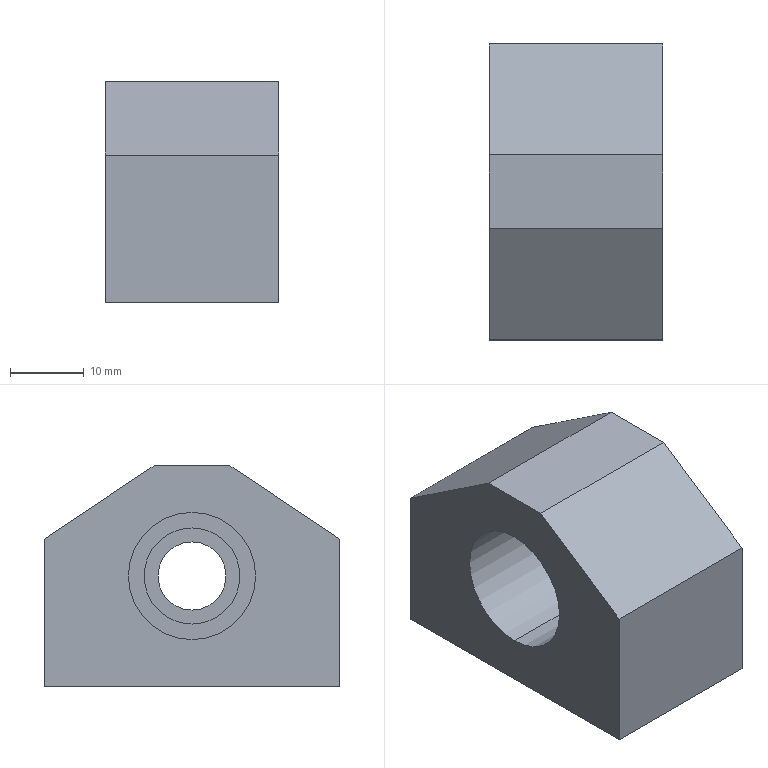Part | SolidWorks | features BaseBody 1 | 1 solid | 22 faces | box 23.5 x 40 x 30 mm | volume 19711 mm3 | plane 12 | cylinder 10 | commonest cylinder face diameters 6 x4 9.2 x2 13 x2 17.2 x2
STEP:
#1=CARTESIAN_POINT('',(896.946,-4295.973,955.371));
#2=VERTEX_POINT('',#1);
#3=CARTESIAN_POINT('',(896.946,-4295.973,964.571));
#4=VERTEX_POINT('',#3);
#5=CARTESIAN_POINT('',(896.946,-4295.973,959.971));
#6=DIRECTION('',(-1.,0.,0.));
#7=DIRECTION('',(0.,0.,1.));
#8=AXIS2_PLACEMENT_3D('',#5,#6,#7);
#9=CIRCLE('',#8,4.6);
#10=EDGE_CURVE('',#2,#4,#9,.T.);
#11=ORIENTED_EDGE('',*,*,#10,.F.);
#12=CARTESIAN_POINT('',(893.946,-4295.973,955.371));
#13=VERTEX_POINT('',#12);
#14=CARTESIAN_POINT('',(851.713,-4295.973,955.371));
#15=DIRECTION('',(-1.,0.,0.));
#16=VECTOR('',#15,1000.);
#17=LINE('',#14,#16);
#18=EDGE_CURVE('',#2,#13,#17,.T.);
#19=ORIENTED_EDGE('',*,*,#18,.T.);
#20=CARTESIAN_POINT('',(893.946,-4295.973,964.571));
#21=VERTEX_POINT('',#20);
#22=CARTESIAN_POINT('',(893.946,-4295.973,959.971));
#23=DIRECTION('',(1.,0.,0.));
#24=DIRECTION('',(0.,0.,1.));
#25=AXIS2_PLACEMENT_3D('',#22,#23,#24);
#26=CIRCLE('',#25,4.6);
#27=EDGE_CURVE('',#21,#13,#26,.T.);
#28=ORIENTED_EDGE('',*,*,#27,.F.);
#29=CARTESIAN_POINT('',(851.713,-4295.973,964.571));
#30=DIRECTION('',(-1.,0.,0.));
#31=VECTOR('',#30,1000.);
#32=LINE('',#29,#31);
#33=EDGE_CURVE('',#4,#21,#32,.T.);
#34=ORIENTED_EDGE('',*,*,#33,.F.);
#35=EDGE_LOOP('',(#11,#19,#28,#34));
#36=FACE_OUTER_BOUND('',#35,.T.);
#37=CARTESIAN_POINT('',(851.713,-4295.973,959.971));
#38=DIRECTION('',(-1.,0.,0.));
#39=DIRECTION('',(0.,0.,1.));
#40=AXIS2_PLACEMENT_3D('',#37,#38,#39);
#41=CYLINDRICAL_SURFACE('',#40,4.6);
#42=ADVANCED_FACE('',(#36),#41,.F.);
#43=CARTESIAN_POINT('',(888.196,-4280.973,944.971));
#44=VERTEX_POINT('',#43);
#45=CARTESIAN_POINT('',(882.196,-4280.973,944.971));
#46=VERTEX_POINT('',#45);
#47=CARTESIAN_POINT('',(885.196,-4280.973,944.971));
#48=DIRECTION('',(0.,0.,-1.));
#49=DIRECTION('',(1.,0.,0.));
#50=AXIS2_PLACEMENT_3D('',#47,#48,#49);
#51=CIRCLE('',#50,3.);
#52=EDGE_CURVE('',#44,#46,#51,.T.);
#53=ORIENTED_EDGE('',*,*,#52,.T.);
#54=CARTESIAN_POINT('',(882.196,-4280.973,959.971));
#55=VERTEX_POINT('',#54);
#56=CARTESIAN_POINT('',(882.196,-4280.973,909.971));
#57=DIRECTION('',(0.,0.,1.));
#58=VECTOR('',#57,1000.);
#59=LINE('',#56,#58);
#60=EDGE_CURVE('',#46,#55,#59,.T.);
#61=ORIENTED_EDGE('',*,*,#60,.T.);
#62=CARTESIAN_POINT('',(888.196,-4280.973,959.971));
#63=VERTEX_POINT('',#62);
#64=CARTESIAN_POINT('',(885.196,-4280.973,959.971));
#65=DIRECTION('',(0.,0.,-1.));
#66=DIRECTION('',(1.,0.,0.));
#67=AXIS2_PLACEMENT_3D('',#64,#65,#66);
#68=CIRCLE('',#67,3.);
#69=EDGE_CURVE('',#63,#55,#68,.T.);
#70=ORIENTED_EDGE('',*,*,#69,.F.);
#71=CARTESIAN_POINT('',(888.196,-4280.973,909.971));
#72=DIRECTION('',(0.,0.,1.));
#73=VECTOR('',#72,1000.);
#74=LINE('',#71,#73);
#75=EDGE_CURVE('',#44,#63,#74,.T.);
#76=ORIENTED_EDGE('',*,*,#75,.F.);
#77=EDGE_LOOP('',(#53,#61,#70,#76));
#78=FACE_OUTER_BOUND('',#77,.T.);
#79=CARTESIAN_POINT('',(885.196,-4280.973,909.971));
#80=DIRECTION('',(0.,0.,1.));
#81=DIRECTION('',(1.,0.,0.));
#82=AXIS2_PLACEMENT_3D('',#79,#80,#81);
#83=CYLINDRICAL_SURFACE('',#82,3.);
#84=ADVANCED_FACE('',(#78),#83,.F.);
#85=CARTESIAN_POINT('',(888.196,-4310.973,959.971));
#86=VERTEX_POINT('',#85);
#87=CARTESIAN_POINT('',(882.196,-4310.973,959.971));
#88=VERTEX_POINT('',#87);
#89=CARTESIAN_POINT('',(885.196,-4310.973,959.971));
#90=DIRECTION('',(0.,0.,-1.));
#91=DIRECTION('',(-1.,0.,0.));
#92=AXIS2_PLACEMENT_3D('',#89,#90,#91);
#93=CIRCLE('',#92,3.);
#94=EDGE_CURVE('',#86,#88,#93,.T.);
#95=ORIENTED_EDGE('',*,*,#94,.F.);
#96=CARTESIAN_POINT('',(888.196,-4310.973,944.971));
#97=VERTEX_POINT('',#96);
#98=CARTESIAN_POINT('',(888.196,-4310.973,909.971));
#99=DIRECTION('',(0.,0.,-1.));
#100=VECTOR('',#99,1000.);
#101=LINE('',#98,#100);
#102=EDGE_CURVE('',#86,#97,#101,.T.);
#103=ORIENTED_EDGE('',*,*,#102,.T.);
#104=CARTESIAN_POINT('',(882.196,-4310.973,944.971));
#105=VERTEX_POINT('',#104);
#106=CARTESIAN_POINT('',(885.196,-4310.973,944.971));
#107=DIRECTION('',(0.,0.,-1.));
#108=DIRECTION('',(-1.,0.,0.));
#109=AXIS2_PLACEMENT_3D('',#106,#107,#108);
#110=CIRCLE('',#109,3.);
#111=EDGE_CURVE('',#97,#105,#110,.T.);
#112=ORIENTED_EDGE('',*,*,#111,.T.);
#113=CARTESIAN_POINT('',(882.196,-4310.973,909.971));
#114=DIRECTION('',(0.,0.,-1.));
#115=VECTOR('',#114,1000.);
#116=LINE('',#113,#115);
#117=EDGE_CURVE('',#88,#105,#116,.T.);
#118=ORIENTED_EDGE('',*,*,#117,.F.);
#119=EDGE_LOOP('',(#95,#103,#112,#118));
#120=FACE_OUTER_BOUND('',#119,.T.);
#121=CARTESIAN_POINT('',(885.196,-4310.973,909.971));
#122=DIRECTION('',(0.,0.,-1.));
#123=DIRECTION('',(-1.,0.,0.));
#124=AXIS2_PLACEMENT_3D('',#121,#122,#123);
#125=CYLINDRICAL_SURFACE('',#124,3.);
#126=ADVANCED_FACE('',(#120),#125,.F.);
#127=CARTESIAN_POINT('',(893.946,-4295.973,966.471));
#128=VERTEX_POINT('',#127);
#129=CARTESIAN_POINT('',(893.946,-4295.973,953.471));
#130=VERTEX_POINT('',#129);
#131=CARTESIAN_POINT('',(893.946,-4295.973,959.971));
#132=DIRECTION('',(1.,0.,0.));
#133=DIRECTION('',(0.,0.,1.));
#134=AXIS2_PLACEMENT_3D('',#131,#132,#133);
#135=CIRCLE('',#134,6.5);
#136=EDGE_CURVE('',#128,#130,#135,.T.);
#137=ORIENTED_EDGE('',*,*,#136,.T.);
#138=CARTESIAN_POINT('',(885.446,-4295.973,953.471));
#139=VERTEX_POINT('',#138);
#140=CARTESIAN_POINT('',(818.946,-4295.973,953.471));
#141=DIRECTION('',(-1.,0.,0.));
#142=VECTOR('',#141,1000.);
#143=LINE('',#140,#142);
#144=EDGE_CURVE('',#130,#139,#143,.T.);
#145=ORIENTED_EDGE('',*,*,#144,.T.);
#146=CARTESIAN_POINT('',(885.446,-4295.973,966.471));
#147=VERTEX_POINT('',#146);
#148=CARTESIAN_POINT('',(885.446,-4295.973,959.971));
#149=DIRECTION('',(1.,0.,0.));
#150=DIRECTION('',(0.,0.,1.));
#151=AXIS2_PLACEMENT_3D('',#148,#149,#150);
#152=CIRCLE('',#151,6.5);
#153=EDGE_CURVE('',#147,#139,#152,.T.);
#154=ORIENTED_EDGE('',*,*,#153,.F.);
#155=CARTESIAN_POINT('',(818.946,-4295.973,966.471));
#156=DIRECTION('',(-1.,0.,0.));
#157=VECTOR('',#156,1000.);
#158=LINE('',#155,#157);
#159=EDGE_CURVE('',#128,#147,#158,.T.);
#160=ORIENTED_EDGE('',*,*,#159,.F.);
#161=EDGE_LOOP('',(#137,#145,#154,#160));
#162=FACE_OUTER_BOUND('',#161,.T.);
#163=CARTESIAN_POINT('',(818.946,-4295.973,959.971));
#164=DIRECTION('',(-1.,0.,0.));
#165=DIRECTION('',(0.,0.,1.));
#166=AXIS2_PLACEMENT_3D('',#163,#164,#165);
#167=CYLINDRICAL_SURFACE('',#166,6.5);
#168=ADVANCED_FACE('',(#162),#167,.F.);
#169=CARTESIAN_POINT('',(885.446,-4295.973,951.371));
#170=VERTEX_POINT('',#169);
#171=CARTESIAN_POINT('',(885.446,-4295.973,968.571));
#172=VERTEX_POINT('',#171);
#173=CARTESIAN_POINT('',(885.446,-4295.973,959.971));
#174=DIRECTION('',(-1.,0.,0.));
#175=DIRECTION('',(0.,0.,1.));
#176=AXIS2_PLACEMENT_3D('',#173,#174,#175);
#177=CIRCLE('',#176,8.6);
#178=EDGE_CURVE('',#170,#172,#177,.T.);
#179=ORIENTED_EDGE('',*,*,#178,.F.);
#180=CARTESIAN_POINT('',(873.446,-4295.973,951.371));
#181=VERTEX_POINT('',#180);
#182=CARTESIAN_POINT('',(783.446,-4295.973,951.371));
#183=DIRECTION('',(-1.,0.,0.));
#184=VECTOR('',#183,1000.);
#185=LINE('',#182,#184);
#186=EDGE_CURVE('',#170,#181,#185,.T.);
#187=ORIENTED_EDGE('',*,*,#186,.T.);
#188=CARTESIAN_POINT('',(873.446,-4295.973,968.571));
#189=VERTEX_POINT('',#188);
#190=CARTESIAN_POINT('',(873.446,-4295.973,959.971));
#191=DIRECTION('',(1.,0.,0.));
#192=DIRECTION('',(0.,0.,1.));
#193=AXIS2_PLACEMENT_3D('',#190,#191,#192);
#194=CIRCLE('',#193,8.6);
#195=EDGE_CURVE('',#189,#181,#194,.T.);
#196=ORIENTED_EDGE('',*,*,#195,.F.);
#197=CARTESIAN_POINT('',(783.446,-4295.973,968.571));
#198=DIRECTION('',(-1.,0.,0.));
#199=VECTOR('',#198,1000.);
#200=LINE('',#197,#199);
#201=EDGE_CURVE('',#172,#189,#200,.T.);
#202=ORIENTED_EDGE('',*,*,#201,.F.);
#203=EDGE_LOOP('',(#179,#187,#196,#202));
#204=FACE_OUTER_BOUND('',#203,.T.);
#205=CARTESIAN_POINT('',(783.446,-4295.973,959.971));
#206=DIRECTION('',(-1.,0.,0.));
#207=DIRECTION('',(0.,0.,1.));
#208=AXIS2_PLACEMENT_3D('',#205,#206,#207);
#209=CYLINDRICAL_SURFACE('',#208,8.6);
#210=ADVANCED_FACE('',(#204),#209,.F.);
#211=CARTESIAN_POINT('',(896.946,-4295.973,959.971));
#212=DIRECTION('',(-1.,0.,0.));
#213=DIRECTION('',(0.,0.,1.));
#214=AXIS2_PLACEMENT_3D('',#211,#212,#213);
#215=CIRCLE('',#214,4.6);
#216=EDGE_CURVE('',#4,#2,#215,.T.);
#217=ORIENTED_EDGE('',*,*,#216,.T.);
#218=ORIENTED_EDGE('',*,*,#10,.T.);
#219=EDGE_LOOP('',(#217,#218));
#220=FACE_BOUND('',#219,.T.);
#221=CARTESIAN_POINT('',(896.946,-4315.973,944.971));
#222=VERTEX_POINT('',#221);
#223=CARTESIAN_POINT('',(896.946,-4275.973,944.971));
#224=VERTEX_POINT('',#223);
#225=CARTESIAN_POINT('',(896.946,-4275.973,944.971));
#226=DIRECTION('',(0.,1.,0.));
#227=VECTOR('',#226,1000.);
#228=LINE('',#225,#227);
#229=EDGE_CURVE('',#222,#224,#228,.T.);
#230=ORIENTED_EDGE('',*,*,#229,.T.);
#231=CARTESIAN_POINT('',(896.946,-4275.973,964.971));
#232=VERTEX_POINT('',#231);
#233=CARTESIAN_POINT('',(896.946,-4275.973,944.971));
#234=DIRECTION('',(0.,0.,1.));
#235=VECTOR('',#234,1000.);
#236=LINE('',#233,#235);
#237=EDGE_CURVE('',#224,#232,#236,.T.);
#238=ORIENTED_EDGE('',*,*,#237,.T.);
#239=CARTESIAN_POINT('',(896.946,-4290.973,974.971));
#240=VERTEX_POINT('',#239);
#241=CARTESIAN_POINT('',(896.946,-4275.973,964.971));
#242=DIRECTION('',(0.,-0.8321,0.5547));
#243=VECTOR('',#242,1000.);
#244=LINE('',#241,#243);
#245=EDGE_CURVE('',#232,#240,#244,.T.);
#246=ORIENTED_EDGE('',*,*,#245,.T.);
#247=CARTESIAN_POINT('',(896.946,-4300.973,974.971));
#248=VERTEX_POINT('',#247);
#249=CARTESIAN_POINT('',(896.946,-4275.973,974.971));
#250=DIRECTION('',(0.,-1.,0.));
#251=VECTOR('',#250,1000.);
#252=LINE('',#249,#251);
#253=EDGE_CURVE('',#240,#248,#252,.T.);
#254=ORIENTED_EDGE('',*,*,#253,.T.);
#255=CARTESIAN_POINT('',(896.946,-4315.973,964.971));
#256=VERTEX_POINT('',#255);
#257=CARTESIAN_POINT('',(896.946,-4300.973,974.971));
#258=DIRECTION('',(0.,-0.8321,-0.5547));
#259=VECTOR('',#258,1000.);
#260=LINE('',#257,#259);
#261=EDGE_CURVE('',#248,#256,#260,.T.);
#262=ORIENTED_EDGE('',*,*,#261,.T.);
#263=CARTESIAN_POINT('',(896.946,-4315.973,944.971));
#264=DIRECTION('',(0.,0.,-1.));
#265=VECTOR('',#264,1000.);
#266=LINE('',#263,#265);
#267=EDGE_CURVE('',#256,#222,#266,.T.);
#268=ORIENTED_EDGE('',*,*,#267,.T.);
#269=EDGE_LOOP('',(#230,#238,#246,#254,#262,#268));
#270=FACE_OUTER_BOUND('',#269,.T.);
#271=CARTESIAN_POINT('',(896.946,-4275.973,944.971));
#272=DIRECTION('',(1.,0.,0.));
#273=DIRECTION('',(0.,0.,-1.));
#274=AXIS2_PLACEMENT_3D('',#271,#272,#273);
#275=PLANE('',#274);
#276=ADVANCED_FACE('',(#220,#270),#275,.T.);
#277=ORIENTED_EDGE('',*,*,#18,.F.);
#278=ORIENTED_EDGE('',*,*,#216,.F.);
#279=ORIENTED_EDGE('',*,*,#33,.T.);
#280=CARTESIAN_POINT('',(893.946,-4295.973,959.971));
#281=DIRECTION('',(1.,0.,0.));
#282=DIRECTION('',(0.,0.,1.));
#283=AXIS2_PLACEMENT_3D('',#280,#281,#282);
#284=CIRCLE('',#283,4.6);
#285=EDGE_CURVE('',#13,#21,#284,.T.);
#286=ORIENTED_EDGE('',*,*,#285,.F.);
#287=EDGE_LOOP('',(#277,#278,#279,#286));
#288=FACE_OUTER_BOUND('',#287,.T.);
#289=CARTESIAN_POINT('',(851.713,-4295.973,959.971));
#290=DIRECTION('',(-1.,0.,0.));
#291=DIRECTION('',(0.,0.,1.));
#292=AXIS2_PLACEMENT_3D('',#289,#290,#291);
#293=CYLINDRICAL_SURFACE('',#292,4.6);
#294=ADVANCED_FACE('',(#288),#293,.F.);
#295=CARTESIAN_POINT('',(873.446,-4275.973,944.971));
#296=VERTEX_POINT('',#295);
#297=CARTESIAN_POINT('',(873.446,-4275.973,944.971));
#298=DIRECTION('',(-1.,0.,0.));
#299=VECTOR('',#298,1000.);
#300=LINE('',#297,#299);
#301=EDGE_CURVE('',#224,#296,#300,.T.);
#302=ORIENTED_EDGE('',*,*,#301,.T.);
#303=CARTESIAN_POINT('',(873.446,-4275.973,964.971));
#304=VERTEX_POINT('',#303);
#305=CARTESIAN_POINT('',(873.446,-4275.973,944.971));
#306=DIRECTION('',(0.,0.,1.));
#307=VECTOR('',#306,1000.);
#308=LINE('',#305,#307);
#309=EDGE_CURVE('',#296,#304,#308,.T.);
#310=ORIENTED_EDGE('',*,*,#309,.T.);
#311=CARTESIAN_POINT('',(873.446,-4275.973,964.971));
#312=DIRECTION('',(1.,0.,0.));
#313=VECTOR('',#312,1000.);
#314=LINE('',#311,#313);
#315=EDGE_CURVE('',#304,#232,#314,.T.);
#316=ORIENTED_EDGE('',*,*,#315,.T.);
#317=ORIENTED_EDGE('',*,*,#237,.F.);
#318=EDGE_LOOP('',(#302,#310,#316,#317));
#319=FACE_OUTER_BOUND('',#318,.T.);
#320=CARTESIAN_POINT('',(873.446,-4275.973,944.971));
#321=DIRECTION('',(0.,1.,0.));
#322=DIRECTION('',(0.,0.,1.));
#323=AXIS2_PLACEMENT_3D('',#320,#321,#322);
#324=PLANE('',#323);
#325=ADVANCED_FACE('',(#319),#324,.T.);
#326=CARTESIAN_POINT('',(873.446,-4315.973,944.971));
#327=VERTEX_POINT('',#326);
#328=CARTESIAN_POINT('',(873.446,-4295.973,944.971));
#329=DIRECTION('',(0.,-1.,0.));
#330=VECTOR('',#329,1000.);
#331=LINE('',#328,#330);
#332=EDGE_CURVE('',#296,#327,#331,.T.);
#333=ORIENTED_EDGE('',*,*,#332,.F.);
#334=ORIENTED_EDGE('',*,*,#301,.F.);
#335=ORIENTED_EDGE('',*,*,#229,.F.);
#336=CARTESIAN_POINT('',(885.196,-4315.973,944.971));
#337=DIRECTION('',(1.,0.,0.));
#338=VECTOR('',#337,1000.);
#339=LINE('',#336,#338);
#340=EDGE_CURVE('',#327,#222,#339,.T.);
#341=ORIENTED_EDGE('',*,*,#340,.F.);
#342=EDGE_LOOP('',(#333,#334,#335,#341));
#343=FACE_OUTER_BOUND('',#342,.T.);
#344=ORIENTED_EDGE('',*,*,#52,.F.);
#345=CARTESIAN_POINT('',(885.196,-4280.973,944.971));
#346=DIRECTION('',(0.,0.,-1.));
#347=DIRECTION('',(1.,0.,0.));
#348=AXIS2_PLACEMENT_3D('',#345,#346,#347);
#349=CIRCLE('',#348,3.);
#350=EDGE_CURVE('',#46,#44,#349,.T.);
#351=ORIENTED_EDGE('',*,*,#350,.F.);
#352=EDGE_LOOP('',(#344,#351));
#353=FACE_BOUND('',#352,.T.);
#354=CARTESIAN_POINT('',(885.196,-4310.973,944.971));
#355=DIRECTION('',(0.,0.,-1.));
#356=DIRECTION('',(-1.,0.,0.));
#357=AXIS2_PLACEMENT_3D('',#354,#355,#356);
#358=CIRCLE('',#357,3.);
#359=EDGE_CURVE('',#105,#97,#358,.T.);
#360=ORIENTED_EDGE('',*,*,#359,.F.);
#361=ORIENTED_EDGE('',*,*,#111,.F.);
#362=EDGE_LOOP('',(#360,#361));
#363=FACE_BOUND('',#362,.T.);
#364=CARTESIAN_POINT('',(885.196,-4295.973,944.971));
#365=DIRECTION('',(0.,0.,1.));
#366=DIRECTION('',(0.,-1.,0.));
#367=AXIS2_PLACEMENT_3D('',#364,#365,#366);
#368=PLANE('',#367);
#369=ADVANCED_FACE('',(#343,#353,#363),#368,.F.);
#370=ORIENTED_EDGE('',*,*,#340,.T.);
#371=ORIENTED_EDGE('',*,*,#267,.F.);
#372=CARTESIAN_POINT('',(873.446,-4315.973,964.971));
#373=VERTEX_POINT('',#372);
#374=CARTESIAN_POINT('',(896.946,-4315.973,964.971));
#375=DIRECTION('',(-1.,0.,0.));
#376=VECTOR('',#375,1000.);
#377=LINE('',#374,#376);
#378=EDGE_CURVE('',#256,#373,#377,.T.);
#379=ORIENTED_EDGE('',*,*,#378,.T.);
#380=CARTESIAN_POINT('',(873.446,-4315.973,944.971));
#381=DIRECTION('',(0.,0.,-1.));
#382=VECTOR('',#381,1000.);
#383=LINE('',#380,#382);
#384=EDGE_CURVE('',#373,#327,#383,.T.);
#385=ORIENTED_EDGE('',*,*,#384,.T.);
#386=EDGE_LOOP('',(#370,#371,#379,#385));
#387=FACE_OUTER_BOUND('',#386,.T.);
#388=CARTESIAN_POINT('',(896.946,-4315.973,944.971));
#389=DIRECTION('',(0.,-1.,0.));
#390=DIRECTION('',(0.,0.,-1.));
#391=AXIS2_PLACEMENT_3D('',#388,#389,#390);
#392=PLANE('',#391);
#393=ADVANCED_FACE('',(#387),#392,.T.);
#394=ORIENTED_EDGE('',*,*,#378,.F.);
#395=ORIENTED_EDGE('',*,*,#261,.F.);
#396=CARTESIAN_POINT('',(873.446,-4300.973,974.971));
#397=VERTEX_POINT('',#396);
#398=CARTESIAN_POINT('',(940.174,-4300.973,974.971));
#399=DIRECTION('',(1.,0.,0.));
#400=VECTOR('',#399,1000.);
#401=LINE('',#398,#400);
#402=EDGE_CURVE('',#397,#248,#401,.T.);
#403=ORIENTED_EDGE('',*,*,#402,.F.);
#404=CARTESIAN_POINT('',(873.446,-4315.973,964.971));
#405=DIRECTION('',(0.,0.8321,0.5547));
#406=VECTOR('',#405,1000.);
#407=LINE('',#404,#406);
#408=EDGE_CURVE('',#373,#397,#407,.T.);
#409=ORIENTED_EDGE('',*,*,#408,.F.);
#410=EDGE_LOOP('',(#394,#395,#403,#409));
#411=FACE_OUTER_BOUND('',#410,.T.);
#412=CARTESIAN_POINT('',(940.174,-4315.973,964.971));
#413=DIRECTION('',(0.,0.5547,-0.8321));
#414=DIRECTION('',(0.,0.8321,0.5547));
#415=AXIS2_PLACEMENT_3D('',#412,#413,#414);
#416=PLANE('',#415);
#417=ADVANCED_FACE('',(#411),#416,.F.);
#418=ORIENTED_EDGE('',*,*,#402,.T.);
#419=ORIENTED_EDGE('',*,*,#253,.F.);
#420=CARTESIAN_POINT('',(873.446,-4290.973,974.971));
#421=VERTEX_POINT('',#420);
#422=CARTESIAN_POINT('',(885.196,-4290.973,974.971));
#423=DIRECTION('',(-1.,0.,0.));
#424=VECTOR('',#423,1000.);
#425=LINE('',#422,#424);
#426=EDGE_CURVE('',#240,#421,#425,.T.);
#427=ORIENTED_EDGE('',*,*,#426,.T.);
#428=CARTESIAN_POINT('',(873.446,-4295.973,974.971));
#429=DIRECTION('',(0.,-1.,0.));
#430=VECTOR('',#429,1000.);
#431=LINE('',#428,#430);
#432=EDGE_CURVE('',#421,#397,#431,.T.);
#433=ORIENTED_EDGE('',*,*,#432,.T.);
#434=EDGE_LOOP('',(#418,#419,#427,#433));
#435=FACE_OUTER_BOUND('',#434,.T.);
#436=CARTESIAN_POINT('',(885.196,-4295.973,974.971));
#437=DIRECTION('',(0.,0.,1.));
#438=DIRECTION('',(0.,-1.,0.));
#439=AXIS2_PLACEMENT_3D('',#436,#437,#438);
#440=PLANE('',#439);
#441=ADVANCED_FACE('',(#435),#440,.T.);
#442=ORIENTED_EDGE('',*,*,#426,.F.);
#443=ORIENTED_EDGE('',*,*,#245,.F.);
#444=ORIENTED_EDGE('',*,*,#315,.F.);
#445=CARTESIAN_POINT('',(873.446,-4275.973,964.971));
#446=DIRECTION('',(0.,0.8321,-0.5547));
#447=VECTOR('',#446,1000.);
#448=LINE('',#445,#447);
#449=EDGE_CURVE('',#421,#304,#448,.T.);
#450=ORIENTED_EDGE('',*,*,#449,.F.);
#451=EDGE_LOOP('',(#442,#443,#444,#450));
#452=FACE_OUTER_BOUND('',#451,.T.);
#453=CARTESIAN_POINT('',(940.174,-4275.973,964.971));
#454=DIRECTION('',(0.,-0.5547,-0.8321));
#455=DIRECTION('',(0.,0.8321,-0.5547));
#456=AXIS2_PLACEMENT_3D('',#453,#454,#455);
#457=PLANE('',#456);
#458=ADVANCED_FACE('',(#452),#457,.F.);
#459=ORIENTED_EDGE('',*,*,#136,.F.);
#460=CARTESIAN_POINT('',(893.946,-4295.973,959.971));
#461=DIRECTION('',(1.,0.,0.));
#462=DIRECTION('',(0.,0.,1.));
#463=AXIS2_PLACEMENT_3D('',#460,#461,#462);
#464=CIRCLE('',#463,6.5);
#465=EDGE_CURVE('',#130,#128,#464,.T.);
#466=ORIENTED_EDGE('',*,*,#465,.F.);
#467=EDGE_LOOP('',(#459,#466));
#468=FACE_OUTER_BOUND('',#467,.T.);
#469=ORIENTED_EDGE('',*,*,#27,.T.);
#470=ORIENTED_EDGE('',*,*,#285,.T.);
#471=EDGE_LOOP('',(#469,#470));
#472=FACE_BOUND('',#471,.T.);
#473=CARTESIAN_POINT('',(893.946,-4295.973,959.971));
#474=DIRECTION('',(1.,0.,0.));
#475=DIRECTION('',(0.,0.,-1.));
#476=AXIS2_PLACEMENT_3D('',#473,#474,#475);
#477=PLANE('',#476);
#478=ADVANCED_FACE('',(#468,#472),#477,.F.);
#479=ORIENTED_EDGE('',*,*,#195,.T.);
#480=CARTESIAN_POINT('',(873.446,-4295.973,959.971));
#481=DIRECTION('',(1.,0.,0.));
#482=DIRECTION('',(0.,0.,1.));
#483=AXIS2_PLACEMENT_3D('',#480,#481,#482);
#484=CIRCLE('',#483,8.6);
#485=EDGE_CURVE('',#181,#189,#484,.T.);
#486=ORIENTED_EDGE('',*,*,#485,.T.);
#487=EDGE_LOOP('',(#479,#486));
#488=FACE_BOUND('',#487,.T.);
#489=ORIENTED_EDGE('',*,*,#408,.T.);
#490=ORIENTED_EDGE('',*,*,#432,.F.);
#491=ORIENTED_EDGE('',*,*,#449,.T.);
#492=ORIENTED_EDGE('',*,*,#309,.F.);
#493=ORIENTED_EDGE('',*,*,#332,.T.);
#494=ORIENTED_EDGE('',*,*,#384,.F.);
#495=EDGE_LOOP('',(#489,#490,#491,#492,#493,#494));
#496=FACE_OUTER_BOUND('',#495,.T.);
#497=CARTESIAN_POINT('',(873.446,-4315.973,944.971));
#498=DIRECTION('',(-1.,0.,0.));
#499=DIRECTION('',(0.,0.,1.));
#500=AXIS2_PLACEMENT_3D('',#497,#498,#499);
#501=PLANE('',#500);
#502=ADVANCED_FACE('',(#488,#496),#501,.T.);
#503=ORIENTED_EDGE('',*,*,#60,.F.);
#504=ORIENTED_EDGE('',*,*,#350,.T.);
#505=ORIENTED_EDGE('',*,*,#75,.T.);
#506=CARTESIAN_POINT('',(885.196,-4280.973,959.971));
#507=DIRECTION('',(0.,0.,-1.));
#508=DIRECTION('',(1.,0.,0.));
#509=AXIS2_PLACEMENT_3D('',#506,#507,#508);
#510=CIRCLE('',#509,3.);
#511=EDGE_CURVE('',#55,#63,#510,.T.);
#512=ORIENTED_EDGE('',*,*,#511,.F.);
#513=EDGE_LOOP('',(#503,#504,#505,#512));
#514=FACE_OUTER_BOUND('',#513,.T.);
#515=CARTESIAN_POINT('',(885.196,-4280.973,909.971));
#516=DIRECTION('',(0.,0.,1.));
#517=DIRECTION('',(1.,0.,0.));
#518=AXIS2_PLACEMENT_3D('',#515,#516,#517);
#519=CYLINDRICAL_SURFACE('',#518,3.);
#520=ADVANCED_FACE('',(#514),#519,.F.);
#521=ORIENTED_EDGE('',*,*,#102,.F.);
#522=CARTESIAN_POINT('',(885.196,-4310.973,959.971));
#523=DIRECTION('',(0.,0.,-1.));
#524=DIRECTION('',(-1.,0.,0.));
#525=AXIS2_PLACEMENT_3D('',#522,#523,#524);
#526=CIRCLE('',#525,3.);
#527=EDGE_CURVE('',#88,#86,#526,.T.);
#528=ORIENTED_EDGE('',*,*,#527,.F.);
#529=ORIENTED_EDGE('',*,*,#117,.T.);
#530=ORIENTED_EDGE('',*,*,#359,.T.);
#531=EDGE_LOOP('',(#521,#528,#529,#530));
#532=FACE_OUTER_BOUND('',#531,.T.);
#533=CARTESIAN_POINT('',(885.196,-4310.973,909.971));
#534=DIRECTION('',(0.,0.,-1.));
#535=DIRECTION('',(-1.,0.,0.));
#536=AXIS2_PLACEMENT_3D('',#533,#534,#535);
#537=CYLINDRICAL_SURFACE('',#536,3.);
#538=ADVANCED_FACE('',(#532),#537,.F.);
#539=ORIENTED_EDGE('',*,*,#144,.F.);
#540=ORIENTED_EDGE('',*,*,#465,.T.);
#541=ORIENTED_EDGE('',*,*,#159,.T.);
#542=CARTESIAN_POINT('',(885.446,-4295.973,959.971));
#543=DIRECTION('',(1.,0.,0.));
#544=DIRECTION('',(0.,0.,1.));
#545=AXIS2_PLACEMENT_3D('',#542,#543,#544);
#546=CIRCLE('',#545,6.5);
#547=EDGE_CURVE('',#139,#147,#546,.T.);
#548=ORIENTED_EDGE('',*,*,#547,.F.);
#549=EDGE_LOOP('',(#539,#540,#541,#548));
#550=FACE_OUTER_BOUND('',#549,.T.);
#551=CARTESIAN_POINT('',(818.946,-4295.973,959.971));
#552=DIRECTION('',(-1.,0.,0.));
#553=DIRECTION('',(0.,0.,1.));
#554=AXIS2_PLACEMENT_3D('',#551,#552,#553);
#555=CYLINDRICAL_SURFACE('',#554,6.5);
#556=ADVANCED_FACE('',(#550),#555,.F.);
#557=ORIENTED_EDGE('',*,*,#186,.F.);
#558=CARTESIAN_POINT('',(885.446,-4295.973,959.971));
#559=DIRECTION('',(-1.,0.,0.));
#560=DIRECTION('',(0.,0.,1.));
#561=AXIS2_PLACEMENT_3D('',#558,#559,#560);
#562=CIRCLE('',#561,8.6);
#563=EDGE_CURVE('',#172,#170,#562,.T.);
#564=ORIENTED_EDGE('',*,*,#563,.F.);
#565=ORIENTED_EDGE('',*,*,#201,.T.);
#566=ORIENTED_EDGE('',*,*,#485,.F.);
#567=EDGE_LOOP('',(#557,#564,#565,#566));
#568=FACE_OUTER_BOUND('',#567,.T.);
#569=CARTESIAN_POINT('',(783.446,-4295.973,959.971));
#570=DIRECTION('',(-1.,0.,0.));
#571=DIRECTION('',(0.,0.,1.));
#572=AXIS2_PLACEMENT_3D('',#569,#570,#571);
#573=CYLINDRICAL_SURFACE('',#572,8.6);
#574=ADVANCED_FACE('',(#568),#573,.F.);
#575=ORIENTED_EDGE('',*,*,#69,.T.);
#576=ORIENTED_EDGE('',*,*,#511,.T.);
#577=EDGE_LOOP('',(#575,#576));
#578=FACE_OUTER_BOUND('',#577,.T.);
#579=CARTESIAN_POINT('',(885.196,-4280.973,959.971));
#580=DIRECTION('',(0.,0.,1.));
#581=DIRECTION('',(1.,0.,0.));
#582=AXIS2_PLACEMENT_3D('',#579,#580,#581);
#583=PLANE('',#582);
#584=ADVANCED_FACE('',(#578),#583,.F.);
#585=ORIENTED_EDGE('',*,*,#527,.T.);
#586=ORIENTED_EDGE('',*,*,#94,.T.);
#587=EDGE_LOOP('',(#585,#586));
#588=FACE_OUTER_BOUND('',#587,.T.);
#589=CARTESIAN_POINT('',(885.196,-4310.973,959.971));
#590=DIRECTION('',(0.,0.,1.));
#591=DIRECTION('',(1.,0.,0.));
#592=AXIS2_PLACEMENT_3D('',#589,#590,#591);
#593=PLANE('',#592);
#594=ADVANCED_FACE('',(#588),#593,.F.);
#595=ORIENTED_EDGE('',*,*,#563,.T.);
#596=ORIENTED_EDGE('',*,*,#178,.T.);
#597=EDGE_LOOP('',(#595,#596));
#598=FACE_OUTER_BOUND('',#597,.T.);
#599=ORIENTED_EDGE('',*,*,#153,.T.);
#600=ORIENTED_EDGE('',*,*,#547,.T.);
#601=EDGE_LOOP('',(#599,#600));
#602=FACE_BOUND('',#601,.T.);
#603=CARTESIAN_POINT('',(885.446,-4295.973,959.971));
#604=DIRECTION('',(1.,0.,0.));
#605=DIRECTION('',(0.,0.,-1.));
#606=AXIS2_PLACEMENT_3D('',#603,#604,#605);
#607=PLANE('',#606);
#608=ADVANCED_FACE('',(#598,#602),#607,.F.);
#609=CLOSED_SHELL('',(#42,#84,#126,#168,#210,#276,#294,#325,#369,#393,#417,#441,#458,#478,#502,#520,#538,#556,#574,#584,#594,#608));
#610=MANIFOLD_SOLID_BREP('',#609);
#611=CARTESIAN_POINT('',(0.,0.,0.));
#612=DIRECTION('',(0.,0.,1.));
#613=DIRECTION('',(1.,0.,0.));
#614=AXIS2_PLACEMENT_3D('',#611,#612,#613);
#615=(LENGTH_UNIT()NAMED_UNIT(*)SI_UNIT(.MILLI.,.METRE.));
#616=UNCERTAINTY_MEASURE_WITH_UNIT(LENGTH_MEASURE(0.00001),#615,'','');
#617=(NAMED_UNIT(*)PLANE_ANGLE_UNIT()SI_UNIT($,.RADIAN.));
#618=(NAMED_UNIT(*)SI_UNIT($,.STERADIAN.)SOLID_ANGLE_UNIT());
#619=(GEOMETRIC_REPRESENTATION_CONTEXT(3)GLOBAL_UNCERTAINTY_ASSIGNED_CONTEXT((#616))GLOBAL_UNIT_ASSIGNED_CONTEXT((#615,#617,#618))REPRESENTATION_CONTEXT('',''));
#620=ADVANCED_BREP_SHAPE_REPRESENTATION('',(#610,#614),#619);